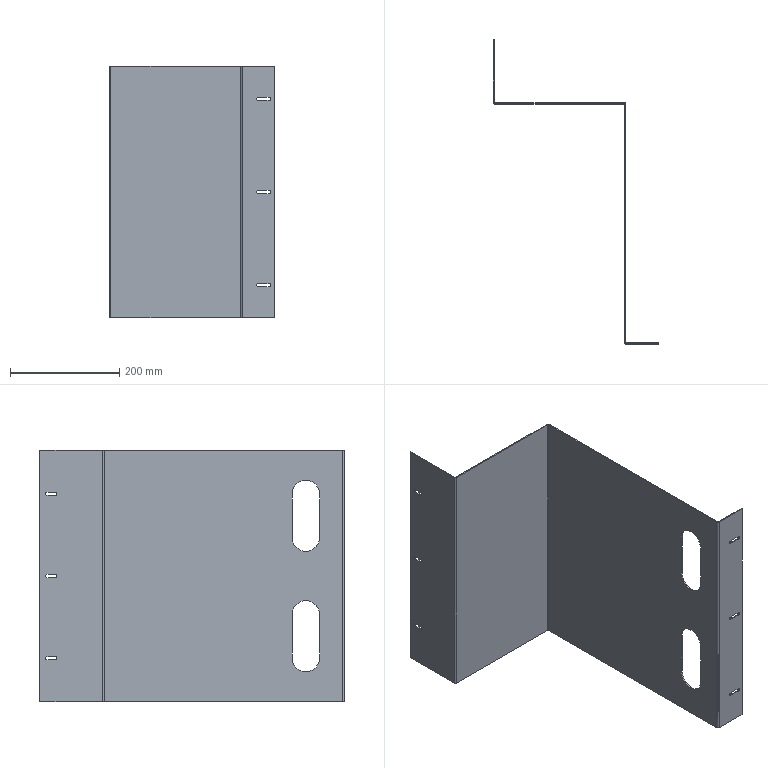Part | STEP file | 11-FG-JX02011 | 1 solid | 65 faces | box 302 x 556 x 460 mm | volume 760169 mm3 | plane 40 | cylinder 25 | commonest cylinder face diameters 5.5 x15 50 x4 1.473 x3 5.473 x3